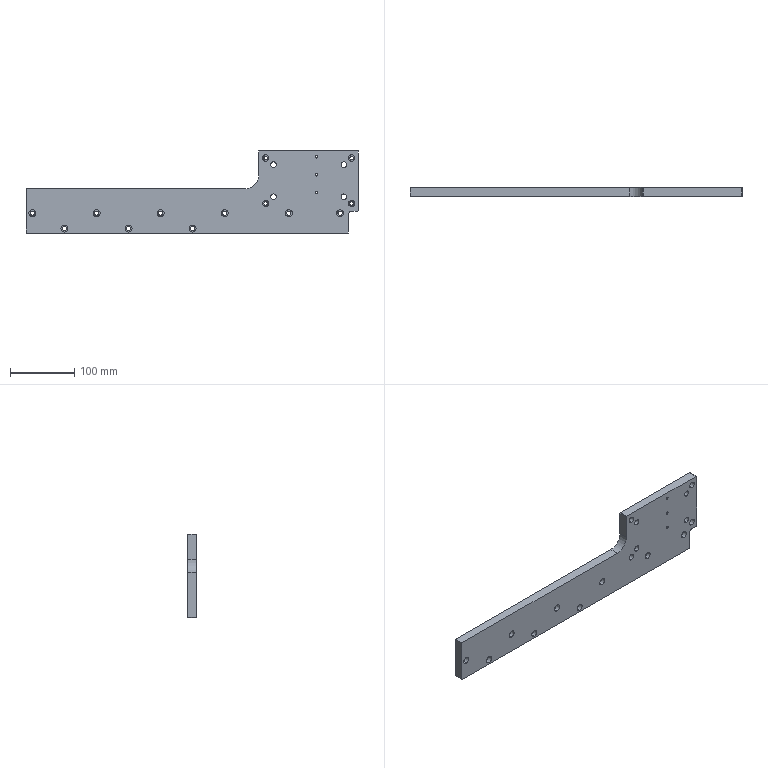Part | SolidWorks | features HoleWzd 5, ICE 3, Chamfer 2, Fillet 2, Extrusion 1 | 1 solid | 96 faces | box 518 x 14 x 130 mm | volume 616033 mm3 | cylinder 68 | plane 28 | commonest cylinder face diameters 6.6 x18 11 x18 10 x9 5.5 x8 9 x8 4.2 x6